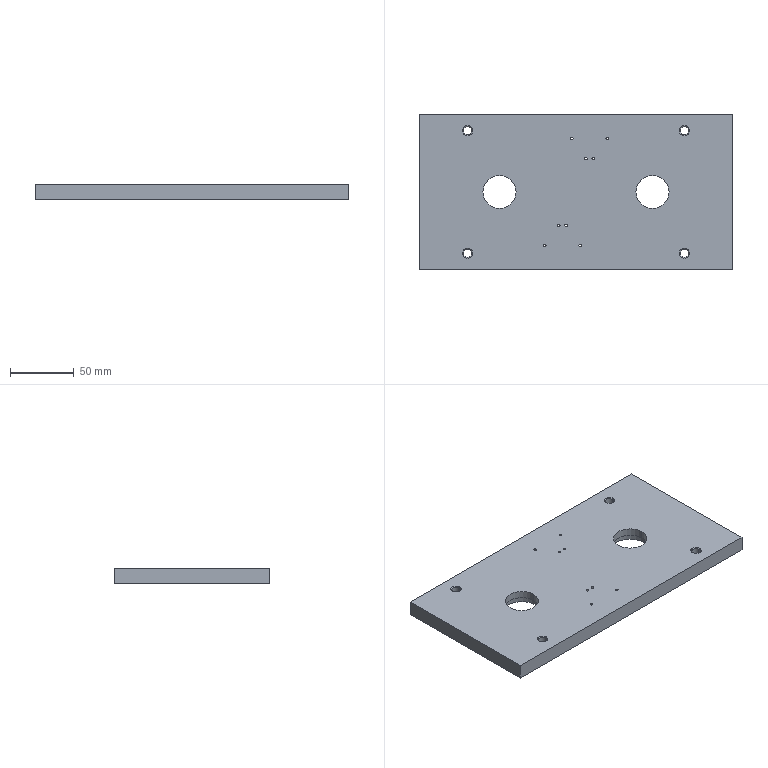Part | STEP file | 9 | 1 solid | 83 faces | box 246 x 122 x 12 mm | volume 330274 mm3 | cylinder 50 | plane 17 | cone 16 | commonest cylinder face diameters 2 x16 3.2 x16 6.647 x8 26 x4 32 x4 50 x2